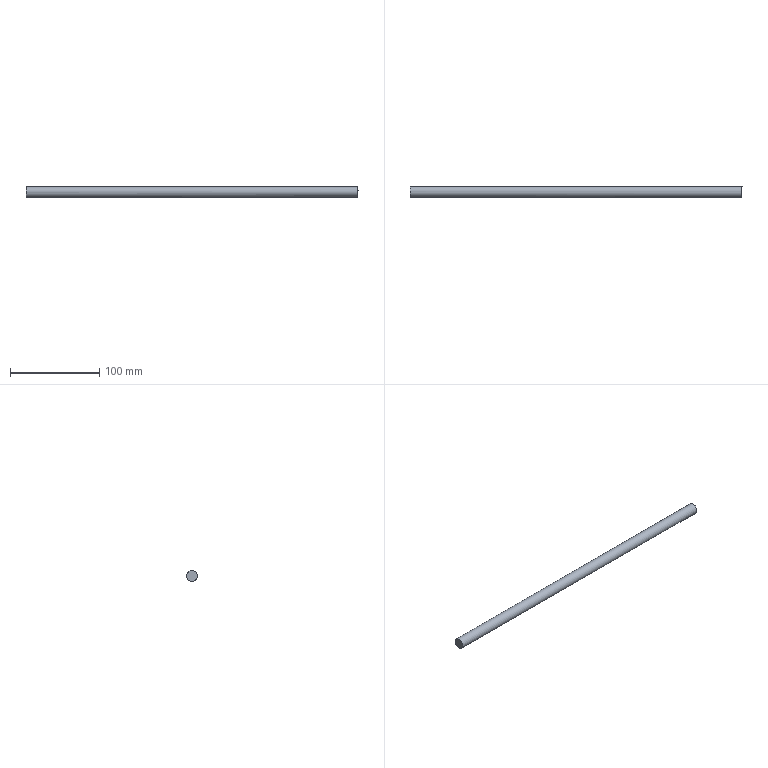Part | STEP file | solid 186 | 1 solid | 4 faces | box 371.47 x 12.005 x 12 mm | volume 41921 mm3 | plane 2 | cylinder 1 | spline 1 | commonest cylinder face diameters 12 x1